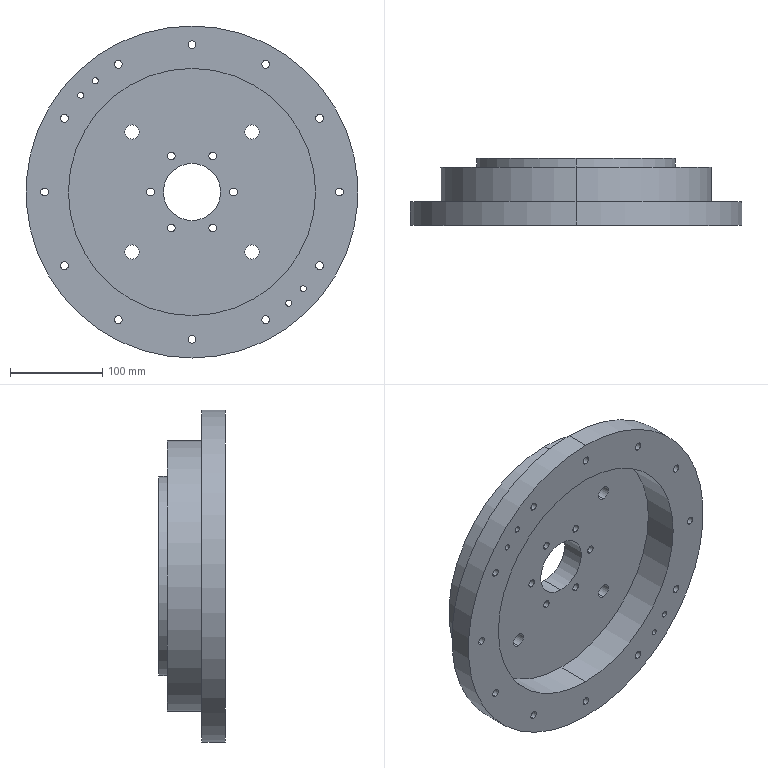Part | STEP file | 1 solid | 70 faces | box 360 x 72.5 x 360 mm | volume 3129469 mm3 | cylinder 64 | plane 6 | commonest cylinder face diameters 8.5 x36 6.5 x8 15.5 x8 62 x2 108 x2 215.9 x2